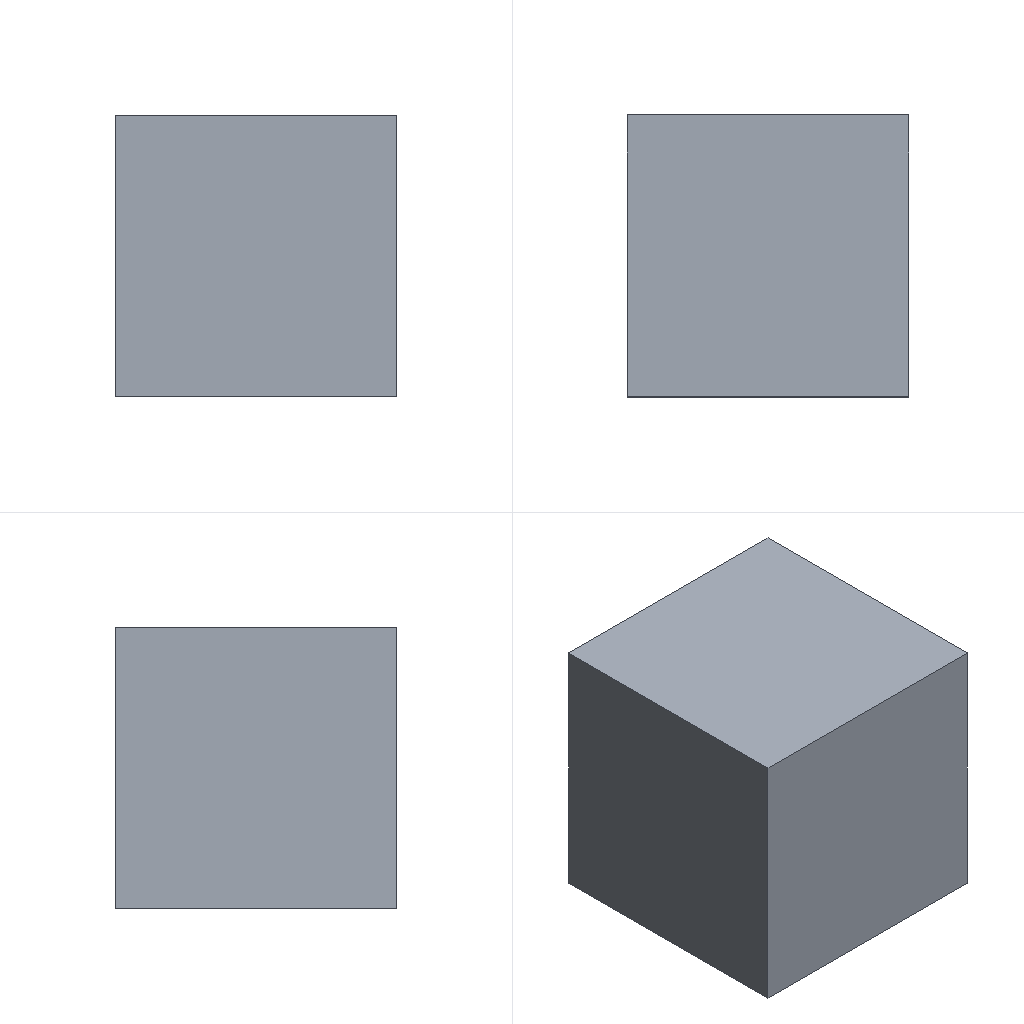Simulation study | abaqus
Set-up summary:
category,name,step,type,value,unit,region
solver,abaqus
solver,version,,,Abaqus/Standard 3DEXPERIENCE R2018x
units,not stated in the deck,,not stated
analysis,deck,,geostatic,geostatic
load_step,geoini,geoini,geostatic
load_step,compress,compress,static
load_step,requested,,,2
mesh,nodes,,,8
mesh,elements,,,1
element_type,C3D8,,solid,1
load,load commands in deck,,count,1
bc,support commands in deck,,count,18
material,SOIL,,in results
check,setup vs results,,match,"per instance, exact: element labels, types and connectivity; labels of the nodes the elements use; coordinates of those nodes at SINGLE_PRECISION in 1 of 1 instance(s)"
Abaqus input file, long lists of numbers shortened:
*Heading
** Job name: ex12-4-O2 Model name: Model-1
** Generated by: Abaqus/CAE 2018
*Preprint, echo=NO, model=NO, history=NO, contact=NO
**
** PARTS
**
*Part, name=Part-1
*Node
      1,           1.,           1.,           1.
      2,           1.,           0.,           1.
** (6 more lines like these left out)
*Element, type=C3D8
1, 5, 6, 8, 7, 1, 2, 4, 3
*Nset, nset=soil, generate
 1,  8,  1
*Elset, elset=soil
 1,
*Nset, nset=_PickedSet5, internal, generate
 1,  8,  1
*Elset, elset=_PickedSet5, internal
 1,
** Section: Section-1
*Solid Section, elset=_PickedSet5, material=soil
,
*End Part
**
**
** ASSEMBLY
**
*Assembly, name=Assembly
**
*Instance, name=Part-1-1, part=Part-1
*End Instance
**
*Nset, nset=Set-5, instance=Part-1-1, generate
 1,  4,  1
*Elset, elset=Set-5, instance=Part-1-1
 1,
*Nset, nset=Set-6, instance=Part-1-1
 1, 2, 5, 6
*Elset, elset=Set-6, instance=Part-1-1
 1,
*Nset, nset=Set-7, instance=Part-1-1, generate
 1,  7,  2
*Elset, elset=Set-7, instance=Part-1-1
 1,
*Nset, nset=_PickedSet6, internal, instance=Part-1-1, generate
 5,  8,  1
*Elset, elset=_PickedSet6, internal, instance=Part-1-1
 1,
*Nset, nset=_PickedSet8, internal, instance=Part-1-1
 3, 4, 7, 8
*Elset, elset=_PickedSet8, internal, instance=Part-1-1
 1,
*Nset, nset=_PickedSet10, internal, instance=Part-1-1, generate
 2,  8,  2
*Elset, elset=_PickedSet10, internal, instance=Part-1-1
 1,
*Nset, nset=_PickedSet12, internal, instance=Part-1-1, generate
 1,  8,  1
*Elset, elset=_PickedSet12, internal, instance=Part-1-1
 1,
*Elset, elset=_Surf-1_S2, internal, instance=Part-1-1
 1,
*Surface, type=ELEMENT, name=Surf-1
_Surf-1_S2, S2
*Elset, elset=_Surf-2_S3, internal, instance=Part-1-1
 1,
*Surface, type=ELEMENT, name=Surf-2
_Surf-2_S3, S3
*End Assembly
**
** MATERIALS
**
*Material, name=soil
*Depvar
      1,
*User Material, constants=7, unsymm
28391.,        0.15,         0.1, 0.0009488,    0.371,       0.114,  0.001283
*INITIAL CONDITIONS, TYPE=SOLUTION
part-1-1.soil,0.0001
**
**
** BOUNDARY CONDITIONS
**
** Name: BC-1 Type: Displacement/Rotation
*Boundary
_PickedSet8, 3, 3
** Name: BC-2 Type: Displacement/Rotation
*Boundary
_PickedSet10, 2, 2
** Name: BC-3 Type: Displacement/Rotation
*Boundary
_PickedSet6, 1, 1
** Name: BC-4 Type: Displacement/Rotation
*Boundary
Set-5, 1, 1
** Name: BC-5 Type: Displacement/Rotation
*Boundary
Set-6, 2, 2
** Name: BC-6 Type: Displacement/Rotation
*Boundary
Set-7, 3, 3
**
** PREDEFINED FIELDS
**
** Name: Predefined Field-1   Type: Stress
*Initial Conditions, type=STRESS
_PickedSet12, 0., 0., 0., 0., 0., 0.
** ----------------------------------------------------------------
**
** STEP: geoini
**
*Step, name=geoini, nlgeom=NO
*Geostatic
**
** BOUNDARY CONDITIONS
**
** Name: BC-1 Type: Displacement/Rotation
*Boundary, op=NEW
_PickedSet8, 3, 3
** Name: BC-2 Type: Displacement/Rotation
*Boundary, op=NEW
_PickedSet10, 2, 2
** Name: BC-3 Type: Displacement/Rotation
*Boundary, op=NEW
_PickedSet6, 1, 1
** Name: BC-4 Type: Displacement/Rotation
*Boundary, op=NEW
Set-5, 1, 1
** Name: BC-5 Type: Displacement/Rotation
*Boundary, op=NEW
Set-6, 2, 2
** Name: BC-6 Type: Displacement/Rotation
*Boundary, op=NEW
Set-7, 3, 3
**
** OUTPUT REQUESTS
**
*Restart, write, frequency=0
**
** FIELD OUTPUT: F-Output-1
**
*Output, field
*Node Output
U,
*Element Output, directions=YES
LE, S, SDV
**
** HISTORY OUTPUT: H-Output-1
**
*Output, history, variable=PRESELECT
*End Step
** ----------------------------------------------------------------
**
** STEP: compress
**
*Step, name=compress, nlgeom=NO, inc=100000000, unsymm=YES
*Static
0.001, 1., 1e-10, 0.001
**
** BOUNDARY CONDITIONS
**
** Name: BC-1 Type: Displacement/Rotation
*Boundary, op=NEW
_PickedSet8, 3, 3
** Name: BC-2 Type: Displacement/Rotation
*Boundary, op=NEW
_PickedSet10, 2, 2
** Name: BC-3 Type: Displacement/Rotation
*Boundary, op=NEW
_PickedSet6, 1, 1
** Name: BC-4 Type: Displacement/Rotation
*Boundary, op=NEW
Set-5, 1, 1, -0.009
** Name: BC-5 Type: Displacement/Rotation
*Boundary, op=NEW
Set-6, 2, 2
** Name: BC-6 Type: Displacement/Rotation
*Boundary, op=NEW
Set-7, 3, 3
**
** SOLVER CONTROLS
**
*Solver Controls, reset
*Solver Controls
0.05, 1000
**
** OUTPUT REQUESTS
**
*Restart, write, frequency=0
**
** FIELD OUTPUT: F-Output-1
**
*Output, field
*Node Output
U,
*Element Output, directions=YES
LE, S, SDV
**
** HISTORY OUTPUT: H-Output-1
**
*Output, history, variable=PRESELECT
*End Step
Results summary:
result,step,,completed,increments=1 time=1.0/1.0
result,step,,partial,increments=364 time=0.364/1.0
result,analysis,,,static
result,last_loadstep,,,2
result,primary field,,,U